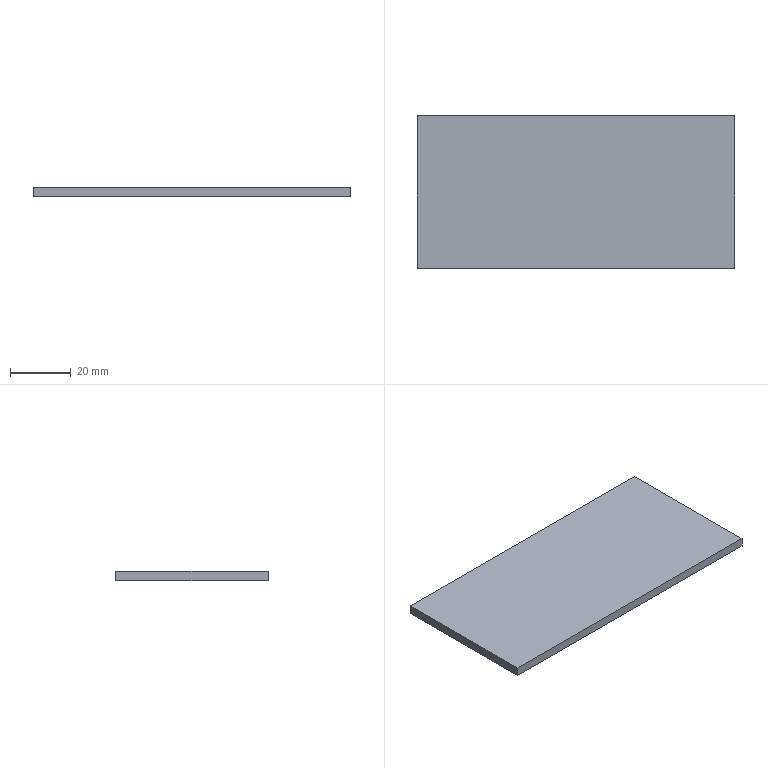Part | STEP file | SX-013-02 | 1 solid | 6 faces | box 104.087 x 50 x 3 mm | volume 15613 mm3 | plane 6
STEP:
#1=CARTESIAN_POINT('',(0.,0.,0.));
#2=DIRECTION('',(0.,0.,1.));
#3=DIRECTION('',(1.,0.,0.));
#4=AXIS2_PLACEMENT_3D('',#1,#2,#3);
#5=CARTESIAN_POINT('',(-49.9,-4385.,0.));
#6=VERTEX_POINT('',#5);
#7=CARTESIAN_POINT('',(-49.9,-4435.,0.));
#8=VERTEX_POINT('',#7);
#9=CARTESIAN_POINT('',(-49.9,-4435.,0.));
#10=DIRECTION('',(0.,-1.,0.));
#11=VECTOR('',#10,1.);
#12=LINE('',#9,#11);
#13=CARTESIAN_POINT('',(-49.9,-4435.,-3.));
#14=DIRECTION('',(-1.,0.,0.));
#15=DIRECTION('',(0.,-1.,0.));
#16=AXIS2_PLACEMENT_3D('',#13,#14,#15);
#17=PLANE('',#16);
#18=CARTESIAN_POINT('',(0.,3.));
#19=DIRECTION('',(1.,0.));
#20=VECTOR('',#19,1.);
#21=LINE('',#18,#20);
#22=(GEOMETRIC_REPRESENTATION_CONTEXT(2)PARAMETRIC_REPRESENTATION_CONTEXT()REPRESENTATION_CONTEXT('',''));
#23=DEFINITIONAL_REPRESENTATION('',(#21),#22);
#24=PCURVE('',#17,#23);
#25=CARTESIAN_POINT('',(0.,0.,0.));
#26=DIRECTION('',(0.,0.,-1.));
#27=DIRECTION('',(-1.,0.,0.));
#28=AXIS2_PLACEMENT_3D('',#25,#26,#27);
#29=PLANE('',#28);
#30=CARTESIAN_POINT('',(49.9,-4435.));
#31=DIRECTION('',(0.,-1.));
#32=VECTOR('',#31,1.);
#33=LINE('',#30,#32);
#34=(GEOMETRIC_REPRESENTATION_CONTEXT(2)PARAMETRIC_REPRESENTATION_CONTEXT()REPRESENTATION_CONTEXT('',''));
#35=DEFINITIONAL_REPRESENTATION('',(#33),#34);
#36=PCURVE('',#29,#35);
#37=SURFACE_CURVE('',#12,(#24,#36),.PCURVE_S1.);
#38=EDGE_CURVE('',#6,#8,#37,.T.);
#39=ORIENTED_EDGE('',*,*,#38,.F.);
#40=CARTESIAN_POINT('',(-49.9,-4385.,-3.));
#41=VERTEX_POINT('',#40);
#42=CARTESIAN_POINT('',(-49.9,-4385.,-3.));
#43=DIRECTION('',(0.,0.,1.));
#44=VECTOR('',#43,1.);
#45=LINE('',#42,#44);
#46=CARTESIAN_POINT('',(-50.,0.));
#47=DIRECTION('',(0.,1.));
#48=VECTOR('',#47,1.);
#49=LINE('',#46,#48);
#50=(GEOMETRIC_REPRESENTATION_CONTEXT(2)PARAMETRIC_REPRESENTATION_CONTEXT()REPRESENTATION_CONTEXT('',''));
#51=DEFINITIONAL_REPRESENTATION('',(#49),#50);
#52=PCURVE('',#17,#51);
#53=CARTESIAN_POINT('',(-49.9,-4385.,-3.));
#54=DIRECTION('',(0.,1.,0.));
#55=DIRECTION('',(0.,0.,1.));
#56=AXIS2_PLACEMENT_3D('',#53,#54,#55);
#57=PLANE('',#56);
#58=CARTESIAN_POINT('',(0.,0.));
#59=DIRECTION('',(1.,0.));
#60=VECTOR('',#59,1.);
#61=LINE('',#58,#60);
#62=(GEOMETRIC_REPRESENTATION_CONTEXT(2)PARAMETRIC_REPRESENTATION_CONTEXT()REPRESENTATION_CONTEXT('',''));
#63=DEFINITIONAL_REPRESENTATION('',(#61),#62);
#64=PCURVE('',#57,#63);
#65=SURFACE_CURVE('',#45,(#52,#64),.PCURVE_S1.);
#66=EDGE_CURVE('',#41,#6,#65,.T.);
#67=ORIENTED_EDGE('',*,*,#66,.F.);
#68=CARTESIAN_POINT('',(-49.9,-4435.,-3.));
#69=VERTEX_POINT('',#68);
#70=CARTESIAN_POINT('',(-49.9,-4435.,-3.));
#71=DIRECTION('',(0.,-1.,0.));
#72=VECTOR('',#71,1.);
#73=LINE('',#70,#72);
#74=CARTESIAN_POINT('',(0.,0.));
#75=DIRECTION('',(1.,0.));
#76=VECTOR('',#75,1.);
#77=LINE('',#74,#76);
#78=(GEOMETRIC_REPRESENTATION_CONTEXT(2)PARAMETRIC_REPRESENTATION_CONTEXT()REPRESENTATION_CONTEXT('',''));
#79=DEFINITIONAL_REPRESENTATION('',(#77),#78);
#80=PCURVE('',#17,#79);
#81=CARTESIAN_POINT('',(0.,0.,-3.));
#82=DIRECTION('',(0.,0.,-1.));
#83=DIRECTION('',(-1.,0.,0.));
#84=AXIS2_PLACEMENT_3D('',#81,#82,#83);
#85=PLANE('',#84);
#86=CARTESIAN_POINT('',(49.9,-4435.));
#87=DIRECTION('',(0.,-1.));
#88=VECTOR('',#87,1.);
#89=LINE('',#86,#88);
#90=(GEOMETRIC_REPRESENTATION_CONTEXT(2)PARAMETRIC_REPRESENTATION_CONTEXT()REPRESENTATION_CONTEXT('',''));
#91=DEFINITIONAL_REPRESENTATION('',(#89),#90);
#92=PCURVE('',#85,#91);
#93=SURFACE_CURVE('',#73,(#80,#92),.PCURVE_S1.);
#94=EDGE_CURVE('',#41,#69,#93,.T.);
#95=ORIENTED_EDGE('',*,*,#94,.T.);
#96=CARTESIAN_POINT('',(-49.9,-4435.,-3.));
#97=DIRECTION('',(0.,0.,1.));
#98=VECTOR('',#97,1.);
#99=LINE('',#96,#98);
#100=CARTESIAN_POINT('',(0.,0.));
#101=DIRECTION('',(0.,1.));
#102=VECTOR('',#101,1.);
#103=LINE('',#100,#102);
#104=(GEOMETRIC_REPRESENTATION_CONTEXT(2)PARAMETRIC_REPRESENTATION_CONTEXT()REPRESENTATION_CONTEXT('',''));
#105=DEFINITIONAL_REPRESENTATION('',(#103),#104);
#106=PCURVE('',#17,#105);
#107=CARTESIAN_POINT('',(-49.9,-4435.,-3.));
#108=DIRECTION('',(0.,-1.,0.));
#109=DIRECTION('',(0.,0.,-1.));
#110=AXIS2_PLACEMENT_3D('',#107,#108,#109);
#111=PLANE('',#110);
#112=CARTESIAN_POINT('',(0.,0.));
#113=DIRECTION('',(-1.,0.));
#114=VECTOR('',#113,1.);
#115=LINE('',#112,#114);
#116=(GEOMETRIC_REPRESENTATION_CONTEXT(2)PARAMETRIC_REPRESENTATION_CONTEXT()REPRESENTATION_CONTEXT('',''));
#117=DEFINITIONAL_REPRESENTATION('',(#115),#116);
#118=PCURVE('',#111,#117);
#119=SURFACE_CURVE('',#99,(#106,#118),.PCURVE_S1.);
#120=EDGE_CURVE('',#69,#8,#119,.T.);
#121=ORIENTED_EDGE('',*,*,#120,.T.);
#122=EDGE_LOOP('',(#39,#67,#95,#121));
#123=FACE_BOUND('',#122,.T.);
#124=ADVANCED_FACE('',(#123),#17,.T.);
#125=CARTESIAN_POINT('',(54.186,-4385.,0.));
#126=VERTEX_POINT('',#125);
#127=CARTESIAN_POINT('',(-49.9,-4385.,0.));
#128=DIRECTION('',(-1.,0.,0.));
#129=VECTOR('',#128,1.);
#130=LINE('',#127,#129);
#131=CARTESIAN_POINT('',(3.,0.));
#132=DIRECTION('',(0.,-1.));
#133=VECTOR('',#132,1.);
#134=LINE('',#131,#133);
#135=(GEOMETRIC_REPRESENTATION_CONTEXT(2)PARAMETRIC_REPRESENTATION_CONTEXT()REPRESENTATION_CONTEXT('',''));
#136=DEFINITIONAL_REPRESENTATION('',(#134),#135);
#137=PCURVE('',#57,#136);
#138=CARTESIAN_POINT('',(49.9,-4385.));
#139=DIRECTION('',(1.,0.));
#140=VECTOR('',#139,1.);
#141=LINE('',#138,#140);
#142=(GEOMETRIC_REPRESENTATION_CONTEXT(2)PARAMETRIC_REPRESENTATION_CONTEXT()REPRESENTATION_CONTEXT('',''));
#143=DEFINITIONAL_REPRESENTATION('',(#141),#142);
#144=PCURVE('',#29,#143);
#145=SURFACE_CURVE('',#130,(#137,#144),.PCURVE_S1.);
#146=EDGE_CURVE('',#126,#6,#145,.T.);
#147=ORIENTED_EDGE('',*,*,#146,.F.);
#148=CARTESIAN_POINT('',(54.186,-4385.,-3.));
#149=VERTEX_POINT('',#148);
#150=CARTESIAN_POINT('',(54.186,-4385.,-3.));
#151=DIRECTION('',(0.,0.,1.));
#152=VECTOR('',#151,1.);
#153=LINE('',#150,#152);
#154=CARTESIAN_POINT('',(0.,104.087));
#155=DIRECTION('',(1.,0.));
#156=VECTOR('',#155,1.);
#157=LINE('',#154,#156);
#158=(GEOMETRIC_REPRESENTATION_CONTEXT(2)PARAMETRIC_REPRESENTATION_CONTEXT()REPRESENTATION_CONTEXT('',''));
#159=DEFINITIONAL_REPRESENTATION('',(#157),#158);
#160=PCURVE('',#57,#159);
#161=CARTESIAN_POINT('',(54.186,-4435.,-3.));
#162=DIRECTION('',(1.,0.,0.));
#163=DIRECTION('',(0.,0.,-1.));
#164=AXIS2_PLACEMENT_3D('',#161,#162,#163);
#165=PLANE('',#164);
#166=CARTESIAN_POINT('',(0.,50.));
#167=DIRECTION('',(-1.,0.));
#168=VECTOR('',#167,1.);
#169=LINE('',#166,#168);
#170=(GEOMETRIC_REPRESENTATION_CONTEXT(2)PARAMETRIC_REPRESENTATION_CONTEXT()REPRESENTATION_CONTEXT('',''));
#171=DEFINITIONAL_REPRESENTATION('',(#169),#170);
#172=PCURVE('',#165,#171);
#173=SURFACE_CURVE('',#153,(#160,#172),.PCURVE_S1.);
#174=EDGE_CURVE('',#149,#126,#173,.T.);
#175=ORIENTED_EDGE('',*,*,#174,.F.);
#176=CARTESIAN_POINT('',(-49.9,-4385.,-3.));
#177=DIRECTION('',(-1.,0.,0.));
#178=VECTOR('',#177,1.);
#179=LINE('',#176,#178);
#180=CARTESIAN_POINT('',(0.,0.));
#181=DIRECTION('',(0.,-1.));
#182=VECTOR('',#181,1.);
#183=LINE('',#180,#182);
#184=(GEOMETRIC_REPRESENTATION_CONTEXT(2)PARAMETRIC_REPRESENTATION_CONTEXT()REPRESENTATION_CONTEXT('',''));
#185=DEFINITIONAL_REPRESENTATION('',(#183),#184);
#186=PCURVE('',#57,#185);
#187=CARTESIAN_POINT('',(49.9,-4385.));
#188=DIRECTION('',(1.,0.));
#189=VECTOR('',#188,1.);
#190=LINE('',#187,#189);
#191=(GEOMETRIC_REPRESENTATION_CONTEXT(2)PARAMETRIC_REPRESENTATION_CONTEXT()REPRESENTATION_CONTEXT('',''));
#192=DEFINITIONAL_REPRESENTATION('',(#190),#191);
#193=PCURVE('',#85,#192);
#194=SURFACE_CURVE('',#179,(#186,#193),.PCURVE_S1.);
#195=EDGE_CURVE('',#149,#41,#194,.T.);
#196=ORIENTED_EDGE('',*,*,#195,.T.);
#197=ORIENTED_EDGE('',*,*,#66,.T.);
#198=EDGE_LOOP('',(#147,#175,#196,#197));
#199=FACE_BOUND('',#198,.T.);
#200=ADVANCED_FACE('',(#199),#57,.T.);
#201=CARTESIAN_POINT('',(54.186,-4435.,0.));
#202=VERTEX_POINT('',#201);
#203=CARTESIAN_POINT('',(54.186,-4435.,0.));
#204=DIRECTION('',(0.,1.,0.));
#205=VECTOR('',#204,1.);
#206=LINE('',#203,#205);
#207=CARTESIAN_POINT('',(-3.,0.));
#208=DIRECTION('',(0.,1.));
#209=VECTOR('',#208,1.);
#210=LINE('',#207,#209);
#211=(GEOMETRIC_REPRESENTATION_CONTEXT(2)PARAMETRIC_REPRESENTATION_CONTEXT()REPRESENTATION_CONTEXT('',''));
#212=DEFINITIONAL_REPRESENTATION('',(#210),#211);
#213=PCURVE('',#165,#212);
#214=CARTESIAN_POINT('',(-54.186,-4435.));
#215=DIRECTION('',(0.,1.));
#216=VECTOR('',#215,1.);
#217=LINE('',#214,#216);
#218=(GEOMETRIC_REPRESENTATION_CONTEXT(2)PARAMETRIC_REPRESENTATION_CONTEXT()REPRESENTATION_CONTEXT('',''));
#219=DEFINITIONAL_REPRESENTATION('',(#217),#218);
#220=PCURVE('',#29,#219);
#221=SURFACE_CURVE('',#206,(#213,#220),.PCURVE_S1.);
#222=EDGE_CURVE('',#202,#126,#221,.T.);
#223=ORIENTED_EDGE('',*,*,#222,.F.);
#224=CARTESIAN_POINT('',(54.186,-4435.,-3.));
#225=VERTEX_POINT('',#224);
#226=CARTESIAN_POINT('',(54.186,-4435.,-3.));
#227=DIRECTION('',(0.,0.,1.));
#228=VECTOR('',#227,1.);
#229=LINE('',#226,#228);
#230=CARTESIAN_POINT('',(0.,0.));
#231=DIRECTION('',(-1.,0.));
#232=VECTOR('',#231,1.);
#233=LINE('',#230,#232);
#234=(GEOMETRIC_REPRESENTATION_CONTEXT(2)PARAMETRIC_REPRESENTATION_CONTEXT()REPRESENTATION_CONTEXT('',''));
#235=DEFINITIONAL_REPRESENTATION('',(#233),#234);
#236=PCURVE('',#165,#235);
#237=CARTESIAN_POINT('',(0.,104.087));
#238=DIRECTION('',(-1.,0.));
#239=VECTOR('',#238,1.);
#240=LINE('',#237,#239);
#241=(GEOMETRIC_REPRESENTATION_CONTEXT(2)PARAMETRIC_REPRESENTATION_CONTEXT()REPRESENTATION_CONTEXT('',''));
#242=DEFINITIONAL_REPRESENTATION('',(#240),#241);
#243=PCURVE('',#111,#242);
#244=SURFACE_CURVE('',#229,(#236,#243),.PCURVE_S1.);
#245=EDGE_CURVE('',#225,#202,#244,.T.);
#246=ORIENTED_EDGE('',*,*,#245,.F.);
#247=CARTESIAN_POINT('',(54.186,-4435.,-3.));
#248=DIRECTION('',(0.,1.,0.));
#249=VECTOR('',#248,1.);
#250=LINE('',#247,#249);
#251=CARTESIAN_POINT('',(0.,0.));
#252=DIRECTION('',(0.,1.));
#253=VECTOR('',#252,1.);
#254=LINE('',#251,#253);
#255=(GEOMETRIC_REPRESENTATION_CONTEXT(2)PARAMETRIC_REPRESENTATION_CONTEXT()REPRESENTATION_CONTEXT('',''));
#256=DEFINITIONAL_REPRESENTATION('',(#254),#255);
#257=PCURVE('',#165,#256);
#258=CARTESIAN_POINT('',(-54.186,-4435.));
#259=DIRECTION('',(0.,1.));
#260=VECTOR('',#259,1.);
#261=LINE('',#258,#260);
#262=(GEOMETRIC_REPRESENTATION_CONTEXT(2)PARAMETRIC_REPRESENTATION_CONTEXT()REPRESENTATION_CONTEXT('',''));
#263=DEFINITIONAL_REPRESENTATION('',(#261),#262);
#264=PCURVE('',#85,#263);
#265=SURFACE_CURVE('',#250,(#257,#264),.PCURVE_S1.);
#266=EDGE_CURVE('',#225,#149,#265,.T.);
#267=ORIENTED_EDGE('',*,*,#266,.T.);
#268=ORIENTED_EDGE('',*,*,#174,.T.);
#269=EDGE_LOOP('',(#223,#246,#267,#268));
#270=FACE_BOUND('',#269,.T.);
#271=ADVANCED_FACE('',(#270),#165,.T.);
#272=CARTESIAN_POINT('',(-49.9,-4435.,0.));
#273=DIRECTION('',(1.,0.,0.));
#274=VECTOR('',#273,1.);
#275=LINE('',#272,#274);
#276=CARTESIAN_POINT('',(-3.,0.));
#277=DIRECTION('',(0.,1.));
#278=VECTOR('',#277,1.);
#279=LINE('',#276,#278);
#280=(GEOMETRIC_REPRESENTATION_CONTEXT(2)PARAMETRIC_REPRESENTATION_CONTEXT()REPRESENTATION_CONTEXT('',''));
#281=DEFINITIONAL_REPRESENTATION('',(#279),#280);
#282=PCURVE('',#111,#281);
#283=CARTESIAN_POINT('',(49.9,-4435.));
#284=DIRECTION('',(-1.,0.));
#285=VECTOR('',#284,1.);
#286=LINE('',#283,#285);
#287=(GEOMETRIC_REPRESENTATION_CONTEXT(2)PARAMETRIC_REPRESENTATION_CONTEXT()REPRESENTATION_CONTEXT('',''));
#288=DEFINITIONAL_REPRESENTATION('',(#286),#287);
#289=PCURVE('',#29,#288);
#290=SURFACE_CURVE('',#275,(#282,#289),.PCURVE_S1.);
#291=EDGE_CURVE('',#8,#202,#290,.T.);
#292=ORIENTED_EDGE('',*,*,#291,.F.);
#293=ORIENTED_EDGE('',*,*,#120,.F.);
#294=CARTESIAN_POINT('',(-49.9,-4435.,-3.));
#295=DIRECTION('',(1.,0.,0.));
#296=VECTOR('',#295,1.);
#297=LINE('',#294,#296);
#298=CARTESIAN_POINT('',(0.,0.));
#299=DIRECTION('',(0.,1.));
#300=VECTOR('',#299,1.);
#301=LINE('',#298,#300);
#302=(GEOMETRIC_REPRESENTATION_CONTEXT(2)PARAMETRIC_REPRESENTATION_CONTEXT()REPRESENTATION_CONTEXT('',''));
#303=DEFINITIONAL_REPRESENTATION('',(#301),#302);
#304=PCURVE('',#111,#303);
#305=CARTESIAN_POINT('',(49.9,-4435.));
#306=DIRECTION('',(-1.,0.));
#307=VECTOR('',#306,1.);
#308=LINE('',#305,#307);
#309=(GEOMETRIC_REPRESENTATION_CONTEXT(2)PARAMETRIC_REPRESENTATION_CONTEXT()REPRESENTATION_CONTEXT('',''));
#310=DEFINITIONAL_REPRESENTATION('',(#308),#309);
#311=PCURVE('',#85,#310);
#312=SURFACE_CURVE('',#297,(#304,#311),.PCURVE_S1.);
#313=EDGE_CURVE('',#69,#225,#312,.T.);
#314=ORIENTED_EDGE('',*,*,#313,.T.);
#315=ORIENTED_EDGE('',*,*,#245,.T.);
#316=EDGE_LOOP('',(#292,#293,#314,#315));
#317=FACE_BOUND('',#316,.T.);
#318=ADVANCED_FACE('',(#317),#111,.T.);
#319=ORIENTED_EDGE('',*,*,#94,.F.);
#320=ORIENTED_EDGE('',*,*,#195,.F.);
#321=ORIENTED_EDGE('',*,*,#266,.F.);
#322=ORIENTED_EDGE('',*,*,#313,.F.);
#323=EDGE_LOOP('',(#319,#320,#321,#322));
#324=FACE_BOUND('',#323,.T.);
#325=ADVANCED_FACE('',(#324),#85,.T.);
#326=ORIENTED_EDGE('',*,*,#38,.T.);
#327=ORIENTED_EDGE('',*,*,#291,.T.);
#328=ORIENTED_EDGE('',*,*,#222,.T.);
#329=ORIENTED_EDGE('',*,*,#146,.T.);
#330=EDGE_LOOP('',(#326,#327,#328,#329));
#331=FACE_BOUND('',#330,.T.);
#332=ADVANCED_FACE('',(#331),#29,.F.);
#333=CLOSED_SHELL('',(#124,#200,#271,#318,#325,#332));
#334=MANIFOLD_SOLID_BREP('',#333);
#335=(LENGTH_UNIT()NAMED_UNIT(*)SI_UNIT(.MILLI.,.METRE.));
#336=UNCERTAINTY_MEASURE_WITH_UNIT(LENGTH_MEASURE(0.0000001),#335,'','');
#337=(NAMED_UNIT(*)PLANE_ANGLE_UNIT()SI_UNIT($,.RADIAN.));
#338=(NAMED_UNIT(*)SI_UNIT($,.STERADIAN.)SOLID_ANGLE_UNIT());
#339=(GEOMETRIC_REPRESENTATION_CONTEXT(3)GLOBAL_UNCERTAINTY_ASSIGNED_CONTEXT((#336))GLOBAL_UNIT_ASSIGNED_CONTEXT((#335,#337,#338))REPRESENTATION_CONTEXT('',''));
#340=ADVANCED_BREP_SHAPE_REPRESENTATION('',(#4,#334),#339);